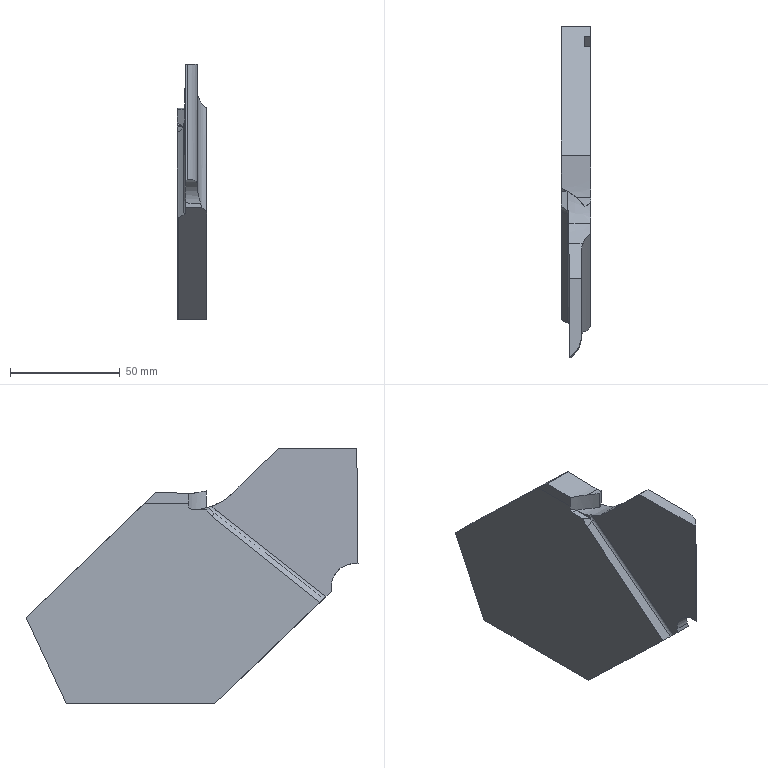Part | Creo | 1 solid | 41 faces | box 13.38 x 151.126 x 116.375 mm | volume 128273 mm3 | plane 23 | cylinder 10 | spline 3 | other 3 | cone 2 | commonest cylinder face diameters 52.261 x2 4.043 x1 21.302 x1 21.315 x1 21.353 x1 22.125 x1